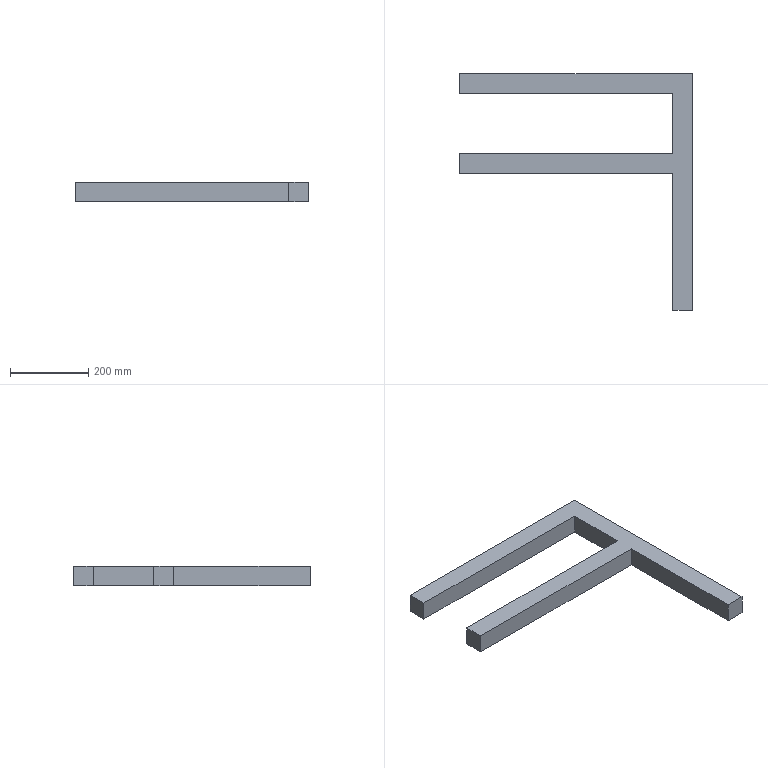Part | SolidWorks | features ICE 10, Cut 1, Extrusion 1 | 1 solid | 12 faces | box 595 x 605 x 50 mm | volume 4237500 mm3 | plane 12
STEP:
#1=CARTESIAN_POINT('',(570.,545.,50.));
#2=VERTEX_POINT('',#1);
#3=CARTESIAN_POINT('',(-25.,545.,50.));
#4=VERTEX_POINT('',#3);
#5=CARTESIAN_POINT('',(570.,545.,50.));
#6=DIRECTION('',(-1.,0.,0.));
#7=VECTOR('',#6,1000.);
#8=LINE('',#5,#7);
#9=EDGE_CURVE('',#2,#4,#8,.T.);
#10=ORIENTED_EDGE('',*,*,#9,.T.);
#11=CARTESIAN_POINT('',(-25.,495.,50.));
#12=VERTEX_POINT('',#11);
#13=CARTESIAN_POINT('',(-25.,495.,50.));
#14=DIRECTION('',(0.,1.,0.));
#15=VECTOR('',#14,1000.);
#16=LINE('',#13,#15);
#17=EDGE_CURVE('',#12,#4,#16,.T.);
#18=ORIENTED_EDGE('',*,*,#17,.F.);
#19=CARTESIAN_POINT('',(520.,495.,50.));
#20=VERTEX_POINT('',#19);
#21=CARTESIAN_POINT('',(520.,495.,50.));
#22=DIRECTION('',(-1.,0.,0.));
#23=VECTOR('',#22,1000.);
#24=LINE('',#21,#23);
#25=EDGE_CURVE('',#20,#12,#24,.T.);
#26=ORIENTED_EDGE('',*,*,#25,.F.);
#27=CARTESIAN_POINT('',(520.,340.,50.));
#28=VERTEX_POINT('',#27);
#29=CARTESIAN_POINT('',(520.,50.,50.));
#30=DIRECTION('',(0.,1.,0.));
#31=VECTOR('',#30,1000.);
#32=LINE('',#29,#31);
#33=EDGE_CURVE('',#28,#20,#32,.T.);
#34=ORIENTED_EDGE('',*,*,#33,.F.);
#35=CARTESIAN_POINT('',(-25.,340.,50.));
#36=VERTEX_POINT('',#35);
#37=CARTESIAN_POINT('',(50.,340.,50.));
#38=DIRECTION('',(1.,0.,0.));
#39=VECTOR('',#38,1000.);
#40=LINE('',#37,#39);
#41=EDGE_CURVE('',#36,#28,#40,.T.);
#42=ORIENTED_EDGE('',*,*,#41,.F.);
#43=CARTESIAN_POINT('',(-25.,290.,50.));
#44=VERTEX_POINT('',#43);
#45=CARTESIAN_POINT('',(-25.,290.,50.));
#46=DIRECTION('',(0.,1.,0.));
#47=VECTOR('',#46,1000.);
#48=LINE('',#45,#47);
#49=EDGE_CURVE('',#44,#36,#48,.T.);
#50=ORIENTED_EDGE('',*,*,#49,.F.);
#51=CARTESIAN_POINT('',(520.,290.,50.));
#52=VERTEX_POINT('',#51);
#53=CARTESIAN_POINT('',(520.,290.,50.));
#54=DIRECTION('',(-1.,0.,0.));
#55=VECTOR('',#54,1000.);
#56=LINE('',#53,#55);
#57=EDGE_CURVE('',#52,#44,#56,.T.);
#58=ORIENTED_EDGE('',*,*,#57,.F.);
#59=CARTESIAN_POINT('',(520.,-60.,50.));
#60=VERTEX_POINT('',#59);
#61=CARTESIAN_POINT('',(520.,50.,50.));
#62=DIRECTION('',(0.,1.,0.));
#63=VECTOR('',#62,1000.);
#64=LINE('',#61,#63);
#65=EDGE_CURVE('',#60,#52,#64,.T.);
#66=ORIENTED_EDGE('',*,*,#65,.F.);
#67=CARTESIAN_POINT('',(570.,-60.,50.));
#68=VERTEX_POINT('',#67);
#69=CARTESIAN_POINT('',(570.,-60.,50.));
#70=DIRECTION('',(-1.,0.,0.));
#71=VECTOR('',#70,1000.);
#72=LINE('',#69,#71);
#73=EDGE_CURVE('',#68,#60,#72,.T.);
#74=ORIENTED_EDGE('',*,*,#73,.F.);
#75=CARTESIAN_POINT('',(570.,0.,50.));
#76=DIRECTION('',(0.,1.,0.));
#77=VECTOR('',#76,1000.);
#78=LINE('',#75,#77);
#79=EDGE_CURVE('',#68,#2,#78,.T.);
#80=ORIENTED_EDGE('',*,*,#79,.T.);
#81=EDGE_LOOP('',(#10,#18,#26,#34,#42,#50,#58,#66,#74,#80));
#82=FACE_OUTER_BOUND('',#81,.T.);
#83=CARTESIAN_POINT('',(0.,0.,50.));
#84=DIRECTION('',(0.,0.,1.));
#85=DIRECTION('',(1.,0.,0.));
#86=AXIS2_PLACEMENT_3D('',#83,#84,#85);
#87=PLANE('',#86);
#88=ADVANCED_FACE('',(#82),#87,.T.);
#89=CARTESIAN_POINT('',(520.,495.,0.));
#90=VERTEX_POINT('',#89);
#91=CARTESIAN_POINT('',(-25.,495.,0.));
#92=VERTEX_POINT('',#91);
#93=CARTESIAN_POINT('',(520.,495.,0.));
#94=DIRECTION('',(-1.,0.,0.));
#95=VECTOR('',#94,1000.);
#96=LINE('',#93,#95);
#97=EDGE_CURVE('',#90,#92,#96,.T.);
#98=ORIENTED_EDGE('',*,*,#97,.T.);
#99=CARTESIAN_POINT('',(-25.,545.,0.));
#100=VERTEX_POINT('',#99);
#101=CARTESIAN_POINT('',(-25.,545.,0.));
#102=DIRECTION('',(0.,-1.,0.));
#103=VECTOR('',#102,1000.);
#104=LINE('',#101,#103);
#105=EDGE_CURVE('',#100,#92,#104,.T.);
#106=ORIENTED_EDGE('',*,*,#105,.F.);
#107=CARTESIAN_POINT('',(570.,545.,0.));
#108=VERTEX_POINT('',#107);
#109=CARTESIAN_POINT('',(570.,545.,0.));
#110=DIRECTION('',(-1.,0.,0.));
#111=VECTOR('',#110,1000.);
#112=LINE('',#109,#111);
#113=EDGE_CURVE('',#108,#100,#112,.T.);
#114=ORIENTED_EDGE('',*,*,#113,.F.);
#115=CARTESIAN_POINT('',(570.,-60.,0.));
#116=VERTEX_POINT('',#115);
#117=CARTESIAN_POINT('',(570.,0.,0.));
#118=DIRECTION('',(0.,1.,0.));
#119=VECTOR('',#118,1000.);
#120=LINE('',#117,#119);
#121=EDGE_CURVE('',#116,#108,#120,.T.);
#122=ORIENTED_EDGE('',*,*,#121,.F.);
#123=CARTESIAN_POINT('',(520.,-60.,0.));
#124=VERTEX_POINT('',#123);
#125=CARTESIAN_POINT('',(520.,-60.,0.));
#126=DIRECTION('',(1.,0.,0.));
#127=VECTOR('',#126,1000.);
#128=LINE('',#125,#127);
#129=EDGE_CURVE('',#124,#116,#128,.T.);
#130=ORIENTED_EDGE('',*,*,#129,.F.);
#131=CARTESIAN_POINT('',(520.,290.,0.));
#132=VERTEX_POINT('',#131);
#133=CARTESIAN_POINT('',(520.,50.,0.));
#134=DIRECTION('',(0.,1.,0.));
#135=VECTOR('',#134,1000.);
#136=LINE('',#133,#135);
#137=EDGE_CURVE('',#124,#132,#136,.T.);
#138=ORIENTED_EDGE('',*,*,#137,.T.);
#139=CARTESIAN_POINT('',(-25.,290.,0.));
#140=VERTEX_POINT('',#139);
#141=CARTESIAN_POINT('',(520.,290.,0.));
#142=DIRECTION('',(-1.,0.,0.));
#143=VECTOR('',#142,1000.);
#144=LINE('',#141,#143);
#145=EDGE_CURVE('',#132,#140,#144,.T.);
#146=ORIENTED_EDGE('',*,*,#145,.T.);
#147=CARTESIAN_POINT('',(-25.,340.,0.));
#148=VERTEX_POINT('',#147);
#149=CARTESIAN_POINT('',(-25.,340.,0.));
#150=DIRECTION('',(0.,-1.,0.));
#151=VECTOR('',#150,1000.);
#152=LINE('',#149,#151);
#153=EDGE_CURVE('',#148,#140,#152,.T.);
#154=ORIENTED_EDGE('',*,*,#153,.F.);
#155=CARTESIAN_POINT('',(520.,340.,0.));
#156=VERTEX_POINT('',#155);
#157=CARTESIAN_POINT('',(50.,340.,0.));
#158=DIRECTION('',(1.,0.,0.));
#159=VECTOR('',#158,1000.);
#160=LINE('',#157,#159);
#161=EDGE_CURVE('',#148,#156,#160,.T.);
#162=ORIENTED_EDGE('',*,*,#161,.T.);
#163=CARTESIAN_POINT('',(520.,50.,0.));
#164=DIRECTION('',(0.,1.,0.));
#165=VECTOR('',#164,1000.);
#166=LINE('',#163,#165);
#167=EDGE_CURVE('',#156,#90,#166,.T.);
#168=ORIENTED_EDGE('',*,*,#167,.T.);
#169=EDGE_LOOP('',(#98,#106,#114,#122,#130,#138,#146,#154,#162,#168));
#170=FACE_OUTER_BOUND('',#169,.T.);
#171=CARTESIAN_POINT('',(0.,0.,0.));
#172=DIRECTION('',(0.,0.,1.));
#173=DIRECTION('',(1.,0.,0.));
#174=AXIS2_PLACEMENT_3D('',#171,#172,#173);
#175=PLANE('',#174);
#176=ADVANCED_FACE('',(#170),#175,.F.);
#177=ORIENTED_EDGE('',*,*,#113,.T.);
#178=CARTESIAN_POINT('',(-25.,545.,50.));
#179=DIRECTION('',(0.,0.,-1.));
#180=VECTOR('',#179,1000.);
#181=LINE('',#178,#180);
#182=EDGE_CURVE('',#4,#100,#181,.T.);
#183=ORIENTED_EDGE('',*,*,#182,.F.);
#184=ORIENTED_EDGE('',*,*,#9,.F.);
#185=CARTESIAN_POINT('',(570.,545.,50.));
#186=DIRECTION('',(0.,0.,-1.));
#187=VECTOR('',#186,1000.);
#188=LINE('',#185,#187);
#189=EDGE_CURVE('',#2,#108,#188,.T.);
#190=ORIENTED_EDGE('',*,*,#189,.T.);
#191=EDGE_LOOP('',(#177,#183,#184,#190));
#192=FACE_OUTER_BOUND('',#191,.T.);
#193=CARTESIAN_POINT('',(570.,545.,50.));
#194=DIRECTION('',(0.,-1.,0.));
#195=DIRECTION('',(0.,0.,-1.));
#196=AXIS2_PLACEMENT_3D('',#193,#194,#195);
#197=PLANE('',#196);
#198=ADVANCED_FACE('',(#192),#197,.F.);
#199=ORIENTED_EDGE('',*,*,#137,.F.);
#200=CARTESIAN_POINT('',(520.,-60.,50.));
#201=DIRECTION('',(0.,0.,-1.));
#202=VECTOR('',#201,1000.);
#203=LINE('',#200,#202);
#204=EDGE_CURVE('',#60,#124,#203,.T.);
#205=ORIENTED_EDGE('',*,*,#204,.F.);
#206=ORIENTED_EDGE('',*,*,#65,.T.);
#207=CARTESIAN_POINT('',(520.,290.,50.));
#208=DIRECTION('',(0.,0.,-1.));
#209=VECTOR('',#208,1000.);
#210=LINE('',#207,#209);
#211=EDGE_CURVE('',#52,#132,#210,.T.);
#212=ORIENTED_EDGE('',*,*,#211,.T.);
#213=EDGE_LOOP('',(#199,#205,#206,#212));
#214=FACE_OUTER_BOUND('',#213,.T.);
#215=CARTESIAN_POINT('',(520.,50.,50.));
#216=DIRECTION('',(-1.,0.,0.));
#217=DIRECTION('',(0.,0.,1.));
#218=AXIS2_PLACEMENT_3D('',#215,#216,#217);
#219=PLANE('',#218);
#220=ADVANCED_FACE('',(#214),#219,.T.);
#221=ORIENTED_EDGE('',*,*,#79,.F.);
#222=CARTESIAN_POINT('',(570.,-60.,0.));
#223=DIRECTION('',(0.,0.,1.));
#224=VECTOR('',#223,1000.);
#225=LINE('',#222,#224);
#226=EDGE_CURVE('',#116,#68,#225,.T.);
#227=ORIENTED_EDGE('',*,*,#226,.F.);
#228=ORIENTED_EDGE('',*,*,#121,.T.);
#229=ORIENTED_EDGE('',*,*,#189,.F.);
#230=EDGE_LOOP('',(#221,#227,#228,#229));
#231=FACE_OUTER_BOUND('',#230,.T.);
#232=CARTESIAN_POINT('',(570.,0.,50.));
#233=DIRECTION('',(-1.,0.,0.));
#234=DIRECTION('',(0.,0.,1.));
#235=AXIS2_PLACEMENT_3D('',#232,#233,#234);
#236=PLANE('',#235);
#237=ADVANCED_FACE('',(#231),#236,.F.);
#238=CARTESIAN_POINT('',(520.,340.,50.));
#239=DIRECTION('',(0.,0.,-1.));
#240=VECTOR('',#239,1000.);
#241=LINE('',#238,#240);
#242=EDGE_CURVE('',#28,#156,#241,.T.);
#243=ORIENTED_EDGE('',*,*,#242,.F.);
#244=ORIENTED_EDGE('',*,*,#33,.T.);
#245=CARTESIAN_POINT('',(520.,495.,50.));
#246=DIRECTION('',(0.,0.,-1.));
#247=VECTOR('',#246,1000.);
#248=LINE('',#245,#247);
#249=EDGE_CURVE('',#20,#90,#248,.T.);
#250=ORIENTED_EDGE('',*,*,#249,.T.);
#251=ORIENTED_EDGE('',*,*,#167,.F.);
#252=EDGE_LOOP('',(#243,#244,#250,#251));
#253=FACE_OUTER_BOUND('',#252,.T.);
#254=CARTESIAN_POINT('',(520.,50.,50.));
#255=DIRECTION('',(-1.,0.,0.));
#256=DIRECTION('',(0.,0.,1.));
#257=AXIS2_PLACEMENT_3D('',#254,#255,#256);
#258=PLANE('',#257);
#259=ADVANCED_FACE('',(#253),#258,.T.);
#260=ORIENTED_EDGE('',*,*,#97,.F.);
#261=ORIENTED_EDGE('',*,*,#249,.F.);
#262=ORIENTED_EDGE('',*,*,#25,.T.);
#263=CARTESIAN_POINT('',(-25.,495.,0.));
#264=DIRECTION('',(0.,0.,1.));
#265=VECTOR('',#264,1000.);
#266=LINE('',#263,#265);
#267=EDGE_CURVE('',#92,#12,#266,.T.);
#268=ORIENTED_EDGE('',*,*,#267,.F.);
#269=EDGE_LOOP('',(#260,#261,#262,#268));
#270=FACE_OUTER_BOUND('',#269,.T.);
#271=CARTESIAN_POINT('',(520.,495.,50.));
#272=DIRECTION('',(0.,-1.,0.));
#273=DIRECTION('',(0.,0.,-1.));
#274=AXIS2_PLACEMENT_3D('',#271,#272,#273);
#275=PLANE('',#274);
#276=ADVANCED_FACE('',(#270),#275,.T.);
#277=ORIENTED_EDGE('',*,*,#145,.F.);
#278=ORIENTED_EDGE('',*,*,#211,.F.);
#279=ORIENTED_EDGE('',*,*,#57,.T.);
#280=CARTESIAN_POINT('',(-25.,290.,0.));
#281=DIRECTION('',(0.,0.,1.));
#282=VECTOR('',#281,1000.);
#283=LINE('',#280,#282);
#284=EDGE_CURVE('',#140,#44,#283,.T.);
#285=ORIENTED_EDGE('',*,*,#284,.F.);
#286=EDGE_LOOP('',(#277,#278,#279,#285));
#287=FACE_OUTER_BOUND('',#286,.T.);
#288=CARTESIAN_POINT('',(520.,290.,50.));
#289=DIRECTION('',(0.,-1.,0.));
#290=DIRECTION('',(0.,0.,-1.));
#291=AXIS2_PLACEMENT_3D('',#288,#289,#290);
#292=PLANE('',#291);
#293=ADVANCED_FACE('',(#287),#292,.T.);
#294=ORIENTED_EDGE('',*,*,#161,.F.);
#295=CARTESIAN_POINT('',(-25.,340.,50.));
#296=DIRECTION('',(0.,0.,-1.));
#297=VECTOR('',#296,1000.);
#298=LINE('',#295,#297);
#299=EDGE_CURVE('',#36,#148,#298,.T.);
#300=ORIENTED_EDGE('',*,*,#299,.F.);
#301=ORIENTED_EDGE('',*,*,#41,.T.);
#302=ORIENTED_EDGE('',*,*,#242,.T.);
#303=EDGE_LOOP('',(#294,#300,#301,#302));
#304=FACE_OUTER_BOUND('',#303,.T.);
#305=CARTESIAN_POINT('',(50.,340.,50.));
#306=DIRECTION('',(0.,1.,0.));
#307=DIRECTION('',(0.,0.,1.));
#308=AXIS2_PLACEMENT_3D('',#305,#306,#307);
#309=PLANE('',#308);
#310=ADVANCED_FACE('',(#304),#309,.T.);
#311=ORIENTED_EDGE('',*,*,#73,.T.);
#312=ORIENTED_EDGE('',*,*,#204,.T.);
#313=ORIENTED_EDGE('',*,*,#129,.T.);
#314=ORIENTED_EDGE('',*,*,#226,.T.);
#315=EDGE_LOOP('',(#311,#312,#313,#314));
#316=FACE_OUTER_BOUND('',#315,.T.);
#317=CARTESIAN_POINT('',(0.,-60.,0.));
#318=DIRECTION('',(0.,-1.,0.));
#319=DIRECTION('',(0.,0.,-1.));
#320=AXIS2_PLACEMENT_3D('',#317,#318,#319);
#321=PLANE('',#320);
#322=ADVANCED_FACE('',(#316),#321,.T.);
#323=ORIENTED_EDGE('',*,*,#182,.T.);
#324=ORIENTED_EDGE('',*,*,#105,.T.);
#325=ORIENTED_EDGE('',*,*,#267,.T.);
#326=ORIENTED_EDGE('',*,*,#17,.T.);
#327=EDGE_LOOP('',(#323,#324,#325,#326));
#328=FACE_OUTER_BOUND('',#327,.T.);
#329=CARTESIAN_POINT('',(-25.,0.,0.));
#330=DIRECTION('',(-1.,0.,0.));
#331=DIRECTION('',(0.,0.,1.));
#332=AXIS2_PLACEMENT_3D('',#329,#330,#331);
#333=PLANE('',#332);
#334=ADVANCED_FACE('',(#328),#333,.T.);
#335=ORIENTED_EDGE('',*,*,#299,.T.);
#336=ORIENTED_EDGE('',*,*,#153,.T.);
#337=ORIENTED_EDGE('',*,*,#284,.T.);
#338=ORIENTED_EDGE('',*,*,#49,.T.);
#339=EDGE_LOOP('',(#335,#336,#337,#338));
#340=FACE_OUTER_BOUND('',#339,.T.);
#341=CARTESIAN_POINT('',(-25.,0.,0.));
#342=DIRECTION('',(-1.,0.,0.));
#343=DIRECTION('',(0.,0.,1.));
#344=AXIS2_PLACEMENT_3D('',#341,#342,#343);
#345=PLANE('',#344);
#346=ADVANCED_FACE('',(#340),#345,.T.);
#347=CLOSED_SHELL('',(#88,#176,#198,#220,#237,#259,#276,#293,#310,#322,#334,#346));
#348=MANIFOLD_SOLID_BREP('',#347);
#349=CARTESIAN_POINT('',(0.,0.,0.));
#350=DIRECTION('',(0.,0.,1.));
#351=DIRECTION('',(1.,0.,0.));
#352=AXIS2_PLACEMENT_3D('',#349,#350,#351);
#353=(LENGTH_UNIT()NAMED_UNIT(*)SI_UNIT(.MILLI.,.METRE.));
#354=UNCERTAINTY_MEASURE_WITH_UNIT(LENGTH_MEASURE(0.00001),#353,'','');
#355=(NAMED_UNIT(*)PLANE_ANGLE_UNIT()SI_UNIT($,.RADIAN.));
#356=(NAMED_UNIT(*)SI_UNIT($,.STERADIAN.)SOLID_ANGLE_UNIT());
#357=(GEOMETRIC_REPRESENTATION_CONTEXT(3)GLOBAL_UNCERTAINTY_ASSIGNED_CONTEXT((#354))GLOBAL_UNIT_ASSIGNED_CONTEXT((#353,#355,#356))REPRESENTATION_CONTEXT('',''));
#358=ADVANCED_BREP_SHAPE_REPRESENTATION('',(#348,#352),#357);